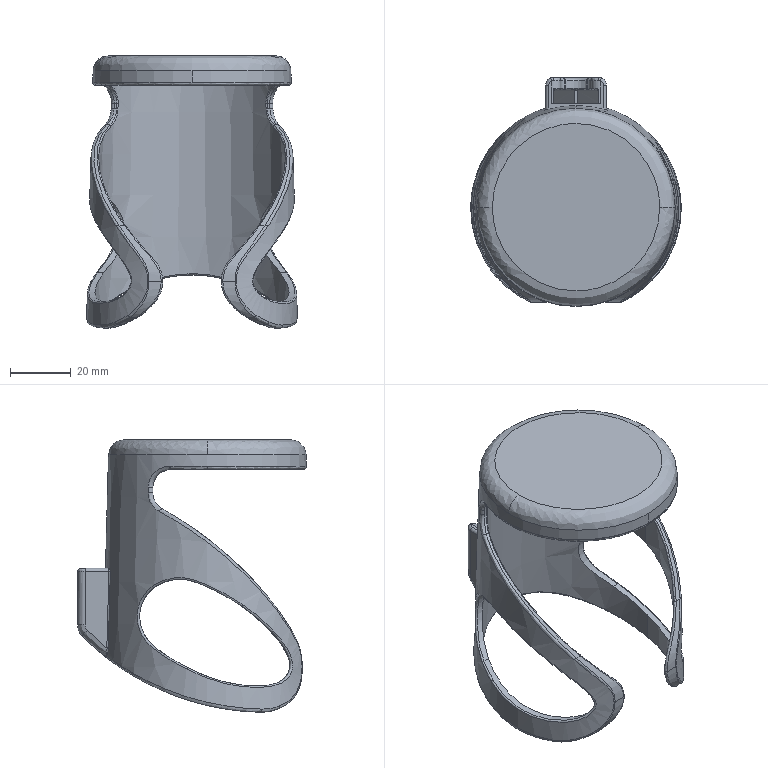Part | SolidWorks | features BaseBody 1 | 1 solid | 152 faces | box 69.285 x 75.31 x 89.558 mm | volume 30202 mm3 | spline 96 | cylinder 34 | plane 16 | cone 6 | commonest cylinder face diameters 2 x7 1 x4 6 x4 12 x4 30 x3 0.999 x2